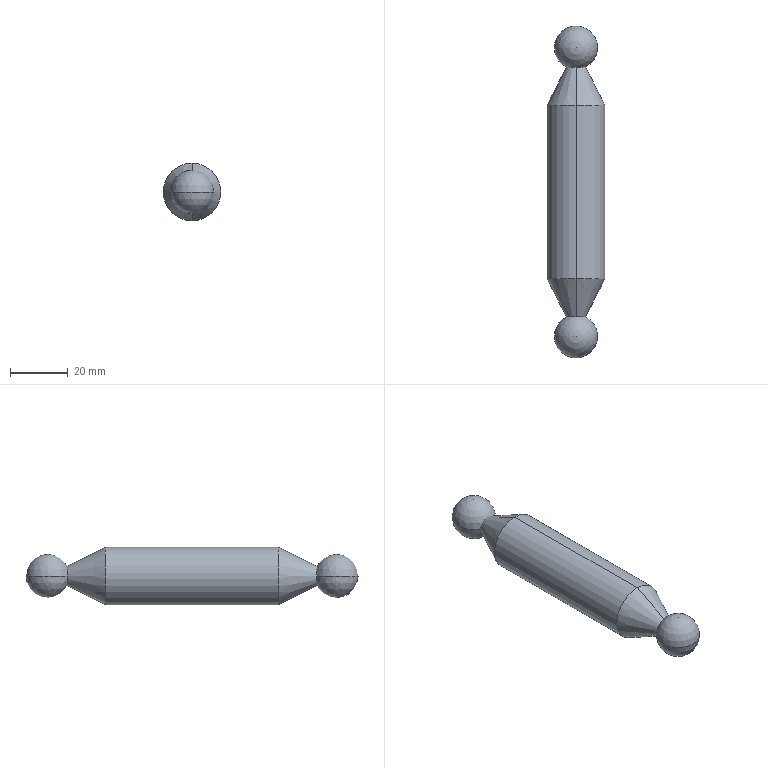Part | SolidWorks | features Revolution 1 | 1 solid | 10 faces | box 20 x 115 x 20 mm | volume 26386 mm3 | sphere 4 | cone 4 | cylinder 2 | commonest cylinder face diameters 20 x2
STEP:
#1=CARTESIAN_POINT('',(0.,6.708,-3.354));
#2=VERTEX_POINT('',#1);
#3=CARTESIAN_POINT('',(3.354,6.708,0.));
#4=VERTEX_POINT('',#3);
#5=CARTESIAN_POINT('',(0.,6.708,0.));
#6=DIRECTION('',(0.,-1.,0.));
#7=DIRECTION('',(0.,0.,-1.));
#8=AXIS2_PLACEMENT_3D('',#5,#6,#7);
#9=CIRCLE('',#8,3.354);
#10=EDGE_CURVE('',#2,#4,#9,.T.);
#11=ORIENTED_EDGE('',*,*,#10,.T.);
#12=CARTESIAN_POINT('',(0.,-7.5,0.));
#13=VERTEX_POINT('',#12);
#14=CARTESIAN_POINT('',(0.,0.,0.));
#15=DIRECTION('',(0.,0.,-1.));
#16=DIRECTION('',(-1.,0.,0.));
#17=AXIS2_PLACEMENT_3D('',#14,#15,#16);
#18=CIRCLE('',#17,7.5);
#19=EDGE_CURVE('',#4,#13,#18,.T.);
#20=ORIENTED_EDGE('',*,*,#19,.T.);
#21=CARTESIAN_POINT('',(-3.354,6.708,0.));
#22=VERTEX_POINT('',#21);
#23=CARTESIAN_POINT('',(0.,0.,0.));
#24=DIRECTION('',(0.,0.,1.));
#25=DIRECTION('',(1.,0.,0.));
#26=AXIS2_PLACEMENT_3D('',#23,#24,#25);
#27=CIRCLE('',#26,7.5);
#28=EDGE_CURVE('',#22,#13,#27,.T.);
#29=ORIENTED_EDGE('',*,*,#28,.F.);
#30=CARTESIAN_POINT('',(0.,6.708,0.));
#31=DIRECTION('',(0.,-1.,0.));
#32=DIRECTION('',(0.,0.,-1.));
#33=AXIS2_PLACEMENT_3D('',#30,#31,#32);
#34=CIRCLE('',#33,3.354);
#35=EDGE_CURVE('',#22,#2,#34,.T.);
#36=ORIENTED_EDGE('',*,*,#35,.T.);
#37=EDGE_LOOP('',(#11,#20,#29,#36));
#38=FACE_OUTER_BOUND('',#37,.T.);
#39=CARTESIAN_POINT('',(0.,0.,0.));
#40=DIRECTION('',(0.,0.,-1.));
#41=DIRECTION('',(-1.,0.,0.));
#42=AXIS2_PLACEMENT_3D('',#39,#40,#41);
#43=SPHERICAL_SURFACE('',#42,7.5);
#44=ADVANCED_FACE('',(#38),#43,.T.);
#45=ORIENTED_EDGE('',*,*,#10,.F.);
#46=CARTESIAN_POINT('',(0.,20.,-10.));
#47=VERTEX_POINT('',#46);
#48=CARTESIAN_POINT('',(0.,20.,-10.));
#49=DIRECTION('',(0.,0.8944,-0.4472));
#50=VECTOR('',#49,1000.);
#51=LINE('',#48,#50);
#52=EDGE_CURVE('',#2,#47,#51,.T.);
#53=ORIENTED_EDGE('',*,*,#52,.T.);
#54=CARTESIAN_POINT('',(0.,20.,10.));
#55=VERTEX_POINT('',#54);
#56=CARTESIAN_POINT('',(0.,20.,0.));
#57=DIRECTION('',(0.,-1.,0.));
#58=DIRECTION('',(0.,0.,-1.));
#59=AXIS2_PLACEMENT_3D('',#56,#57,#58);
#60=CIRCLE('',#59,10.);
#61=EDGE_CURVE('',#47,#55,#60,.T.);
#62=ORIENTED_EDGE('',*,*,#61,.T.);
#63=CARTESIAN_POINT('',(0.,6.708,3.354));
#64=VERTEX_POINT('',#63);
#65=CARTESIAN_POINT('',(0.,20.,10.));
#66=DIRECTION('',(0.,0.8944,0.4472));
#67=VECTOR('',#66,1000.);
#68=LINE('',#65,#67);
#69=EDGE_CURVE('',#64,#55,#68,.T.);
#70=ORIENTED_EDGE('',*,*,#69,.F.);
#71=CARTESIAN_POINT('',(0.,6.708,0.));
#72=DIRECTION('',(0.,-1.,0.));
#73=DIRECTION('',(0.,0.,-1.));
#74=AXIS2_PLACEMENT_3D('',#71,#72,#73);
#75=CIRCLE('',#74,3.354);
#76=EDGE_CURVE('',#4,#64,#75,.T.);
#77=ORIENTED_EDGE('',*,*,#76,.F.);
#78=EDGE_LOOP('',(#45,#53,#62,#70,#77));
#79=FACE_OUTER_BOUND('',#78,.T.);
#80=CARTESIAN_POINT('',(0.,20.,0.));
#81=DIRECTION('',(0.,1.,0.));
#82=DIRECTION('',(0.,0.,1.));
#83=AXIS2_PLACEMENT_3D('',#80,#81,#82);
#84=CONICAL_SURFACE('',#83,10.,0.4636);
#85=ADVANCED_FACE('',(#79),#84,.T.);
#86=CARTESIAN_POINT('',(0.,80.,-10.));
#87=VERTEX_POINT('',#86);
#88=CARTESIAN_POINT('',(0.,80.,10.));
#89=VERTEX_POINT('',#88);
#90=CARTESIAN_POINT('',(0.,80.,0.));
#91=DIRECTION('',(0.,-1.,0.));
#92=DIRECTION('',(0.,0.,-1.));
#93=AXIS2_PLACEMENT_3D('',#90,#91,#92);
#94=CIRCLE('',#93,10.);
#95=EDGE_CURVE('',#87,#89,#94,.T.);
#96=ORIENTED_EDGE('',*,*,#95,.T.);
#97=CARTESIAN_POINT('',(0.,-7.5,10.));
#98=DIRECTION('',(0.,-1.,0.));
#99=VECTOR('',#98,1000.);
#100=LINE('',#97,#99);
#101=EDGE_CURVE('',#89,#55,#100,.T.);
#102=ORIENTED_EDGE('',*,*,#101,.T.);
#103=ORIENTED_EDGE('',*,*,#61,.F.);
#104=CARTESIAN_POINT('',(0.,-7.5,-10.));
#105=DIRECTION('',(0.,-1.,0.));
#106=VECTOR('',#105,1000.);
#107=LINE('',#104,#106);
#108=EDGE_CURVE('',#87,#47,#107,.T.);
#109=ORIENTED_EDGE('',*,*,#108,.F.);
#110=EDGE_LOOP('',(#96,#102,#103,#109));
#111=FACE_OUTER_BOUND('',#110,.T.);
#112=CARTESIAN_POINT('',(0.,-7.5,0.));
#113=DIRECTION('',(0.,-1.,0.));
#114=DIRECTION('',(0.,0.,-1.));
#115=AXIS2_PLACEMENT_3D('',#112,#113,#114);
#116=CYLINDRICAL_SURFACE('',#115,10.);
#117=ADVANCED_FACE('',(#111),#116,.T.);
#118=CARTESIAN_POINT('',(3.354,93.292,0.));
#119=VERTEX_POINT('',#118);
#120=CARTESIAN_POINT('',(0.,93.292,3.354));
#121=VERTEX_POINT('',#120);
#122=CARTESIAN_POINT('',(0.,93.292,0.));
#123=DIRECTION('',(0.,-1.,0.));
#124=DIRECTION('',(0.,0.,-1.));
#125=AXIS2_PLACEMENT_3D('',#122,#123,#124);
#126=CIRCLE('',#125,3.354);
#127=EDGE_CURVE('',#119,#121,#126,.T.);
#128=ORIENTED_EDGE('',*,*,#127,.T.);
#129=CARTESIAN_POINT('',(0.,93.292,3.354));
#130=DIRECTION('',(0.,-0.8944,0.4472));
#131=VECTOR('',#130,1000.);
#132=LINE('',#129,#131);
#133=EDGE_CURVE('',#121,#89,#132,.T.);
#134=ORIENTED_EDGE('',*,*,#133,.T.);
#135=ORIENTED_EDGE('',*,*,#95,.F.);
#136=CARTESIAN_POINT('',(0.,93.292,-3.354));
#137=VERTEX_POINT('',#136);
#138=CARTESIAN_POINT('',(0.,93.292,-3.354));
#139=DIRECTION('',(0.,-0.8944,-0.4472));
#140=VECTOR('',#139,1000.);
#141=LINE('',#138,#140);
#142=EDGE_CURVE('',#137,#87,#141,.T.);
#143=ORIENTED_EDGE('',*,*,#142,.F.);
#144=CARTESIAN_POINT('',(0.,93.292,0.));
#145=DIRECTION('',(0.,-1.,0.));
#146=DIRECTION('',(0.,0.,-1.));
#147=AXIS2_PLACEMENT_3D('',#144,#145,#146);
#148=CIRCLE('',#147,3.354);
#149=EDGE_CURVE('',#137,#119,#148,.T.);
#150=ORIENTED_EDGE('',*,*,#149,.T.);
#151=EDGE_LOOP('',(#128,#134,#135,#143,#150));
#152=FACE_OUTER_BOUND('',#151,.T.);
#153=CARTESIAN_POINT('',(0.,93.292,0.));
#154=DIRECTION('',(0.,-1.,0.));
#155=DIRECTION('',(0.,0.,-1.));
#156=AXIS2_PLACEMENT_3D('',#153,#154,#155);
#157=CONICAL_SURFACE('',#156,3.354,0.4636);
#158=ADVANCED_FACE('',(#152),#157,.T.);
#159=CARTESIAN_POINT('',(0.,107.5,0.));
#160=VERTEX_POINT('',#159);
#161=CARTESIAN_POINT('',(-3.354,93.292,0.));
#162=VERTEX_POINT('',#161);
#163=CARTESIAN_POINT('',(0.,100.,0.));
#164=DIRECTION('',(0.,0.,1.));
#165=DIRECTION('',(1.,0.,0.));
#166=AXIS2_PLACEMENT_3D('',#163,#164,#165);
#167=CIRCLE('',#166,7.5);
#168=EDGE_CURVE('',#160,#162,#167,.T.);
#169=ORIENTED_EDGE('',*,*,#168,.F.);
#170=CARTESIAN_POINT('',(0.,100.,0.));
#171=DIRECTION('',(0.,0.,-1.));
#172=DIRECTION('',(-1.,0.,0.));
#173=AXIS2_PLACEMENT_3D('',#170,#171,#172);
#174=CIRCLE('',#173,7.5);
#175=EDGE_CURVE('',#160,#119,#174,.T.);
#176=ORIENTED_EDGE('',*,*,#175,.T.);
#177=ORIENTED_EDGE('',*,*,#149,.F.);
#178=CARTESIAN_POINT('',(0.,93.292,0.));
#179=DIRECTION('',(0.,-1.,0.));
#180=DIRECTION('',(0.,0.,-1.));
#181=AXIS2_PLACEMENT_3D('',#178,#179,#180);
#182=CIRCLE('',#181,3.354);
#183=EDGE_CURVE('',#162,#137,#182,.T.);
#184=ORIENTED_EDGE('',*,*,#183,.F.);
#185=EDGE_LOOP('',(#169,#176,#177,#184));
#186=FACE_OUTER_BOUND('',#185,.T.);
#187=CARTESIAN_POINT('',(0.,100.,0.));
#188=DIRECTION('',(0.,0.,-1.));
#189=DIRECTION('',(-1.,0.,0.));
#190=AXIS2_PLACEMENT_3D('',#187,#188,#189);
#191=SPHERICAL_SURFACE('',#190,7.5);
#192=ADVANCED_FACE('',(#186),#191,.T.);
#193=ORIENTED_EDGE('',*,*,#175,.F.);
#194=ORIENTED_EDGE('',*,*,#168,.T.);
#195=CARTESIAN_POINT('',(0.,93.292,0.));
#196=DIRECTION('',(0.,-1.,0.));
#197=DIRECTION('',(0.,0.,-1.));
#198=AXIS2_PLACEMENT_3D('',#195,#196,#197);
#199=CIRCLE('',#198,3.354);
#200=EDGE_CURVE('',#121,#162,#199,.T.);
#201=ORIENTED_EDGE('',*,*,#200,.F.);
#202=ORIENTED_EDGE('',*,*,#127,.F.);
#203=EDGE_LOOP('',(#193,#194,#201,#202));
#204=FACE_OUTER_BOUND('',#203,.T.);
#205=CARTESIAN_POINT('',(0.,100.,0.));
#206=DIRECTION('',(0.,0.,-1.));
#207=DIRECTION('',(-1.,0.,0.));
#208=AXIS2_PLACEMENT_3D('',#205,#206,#207);
#209=SPHERICAL_SURFACE('',#208,7.5);
#210=ADVANCED_FACE('',(#204),#209,.T.);
#211=ORIENTED_EDGE('',*,*,#133,.F.);
#212=ORIENTED_EDGE('',*,*,#200,.T.);
#213=ORIENTED_EDGE('',*,*,#183,.T.);
#214=ORIENTED_EDGE('',*,*,#142,.T.);
#215=CARTESIAN_POINT('',(0.,80.,0.));
#216=DIRECTION('',(0.,-1.,0.));
#217=DIRECTION('',(0.,0.,-1.));
#218=AXIS2_PLACEMENT_3D('',#215,#216,#217);
#219=CIRCLE('',#218,10.);
#220=EDGE_CURVE('',#89,#87,#219,.T.);
#221=ORIENTED_EDGE('',*,*,#220,.F.);
#222=EDGE_LOOP('',(#211,#212,#213,#214,#221));
#223=FACE_OUTER_BOUND('',#222,.T.);
#224=CARTESIAN_POINT('',(0.,93.292,0.));
#225=DIRECTION('',(0.,-1.,0.));
#226=DIRECTION('',(0.,0.,-1.));
#227=AXIS2_PLACEMENT_3D('',#224,#225,#226);
#228=CONICAL_SURFACE('',#227,3.354,0.4636);
#229=ADVANCED_FACE('',(#223),#228,.T.);
#230=ORIENTED_EDGE('',*,*,#101,.F.);
#231=ORIENTED_EDGE('',*,*,#220,.T.);
#232=ORIENTED_EDGE('',*,*,#108,.T.);
#233=CARTESIAN_POINT('',(0.,20.,0.));
#234=DIRECTION('',(0.,-1.,0.));
#235=DIRECTION('',(0.,0.,-1.));
#236=AXIS2_PLACEMENT_3D('',#233,#234,#235);
#237=CIRCLE('',#236,10.);
#238=EDGE_CURVE('',#55,#47,#237,.T.);
#239=ORIENTED_EDGE('',*,*,#238,.F.);
#240=EDGE_LOOP('',(#230,#231,#232,#239));
#241=FACE_OUTER_BOUND('',#240,.T.);
#242=CARTESIAN_POINT('',(0.,-7.5,0.));
#243=DIRECTION('',(0.,-1.,0.));
#244=DIRECTION('',(0.,0.,-1.));
#245=AXIS2_PLACEMENT_3D('',#242,#243,#244);
#246=CYLINDRICAL_SURFACE('',#245,10.);
#247=ADVANCED_FACE('',(#241),#246,.T.);
#248=ORIENTED_EDGE('',*,*,#52,.F.);
#249=ORIENTED_EDGE('',*,*,#35,.F.);
#250=CARTESIAN_POINT('',(0.,6.708,0.));
#251=DIRECTION('',(0.,-1.,0.));
#252=DIRECTION('',(0.,0.,-1.));
#253=AXIS2_PLACEMENT_3D('',#250,#251,#252);
#254=CIRCLE('',#253,3.354);
#255=EDGE_CURVE('',#64,#22,#254,.T.);
#256=ORIENTED_EDGE('',*,*,#255,.F.);
#257=ORIENTED_EDGE('',*,*,#69,.T.);
#258=ORIENTED_EDGE('',*,*,#238,.T.);
#259=EDGE_LOOP('',(#248,#249,#256,#257,#258));
#260=FACE_OUTER_BOUND('',#259,.T.);
#261=CARTESIAN_POINT('',(0.,20.,0.));
#262=DIRECTION('',(0.,1.,0.));
#263=DIRECTION('',(0.,0.,1.));
#264=AXIS2_PLACEMENT_3D('',#261,#262,#263);
#265=CONICAL_SURFACE('',#264,10.,0.4636);
#266=ADVANCED_FACE('',(#260),#265,.T.);
#267=ORIENTED_EDGE('',*,*,#19,.F.);
#268=ORIENTED_EDGE('',*,*,#76,.T.);
#269=ORIENTED_EDGE('',*,*,#255,.T.);
#270=ORIENTED_EDGE('',*,*,#28,.T.);
#271=EDGE_LOOP('',(#267,#268,#269,#270));
#272=FACE_OUTER_BOUND('',#271,.T.);
#273=CARTESIAN_POINT('',(0.,0.,0.));
#274=DIRECTION('',(0.,0.,-1.));
#275=DIRECTION('',(-1.,0.,0.));
#276=AXIS2_PLACEMENT_3D('',#273,#274,#275);
#277=SPHERICAL_SURFACE('',#276,7.5);
#278=ADVANCED_FACE('',(#272),#277,.T.);
#279=CLOSED_SHELL('',(#44,#85,#117,#158,#192,#210,#229,#247,#266,#278));
#280=MANIFOLD_SOLID_BREP('',#279);
#281=CARTESIAN_POINT('',(0.,0.,0.));
#282=DIRECTION('',(0.,0.,1.));
#283=DIRECTION('',(1.,0.,0.));
#284=AXIS2_PLACEMENT_3D('',#281,#282,#283);
#285=(LENGTH_UNIT()NAMED_UNIT(*)SI_UNIT(.MILLI.,.METRE.));
#286=UNCERTAINTY_MEASURE_WITH_UNIT(LENGTH_MEASURE(0.00001),#285,'','');
#287=(NAMED_UNIT(*)PLANE_ANGLE_UNIT()SI_UNIT($,.RADIAN.));
#288=(NAMED_UNIT(*)SI_UNIT($,.STERADIAN.)SOLID_ANGLE_UNIT());
#289=(GEOMETRIC_REPRESENTATION_CONTEXT(3)GLOBAL_UNCERTAINTY_ASSIGNED_CONTEXT((#286))GLOBAL_UNIT_ASSIGNED_CONTEXT((#285,#287,#288))REPRESENTATION_CONTEXT('',''));
#290=ADVANCED_BREP_SHAPE_REPRESENTATION('',(#280,#284),#289);